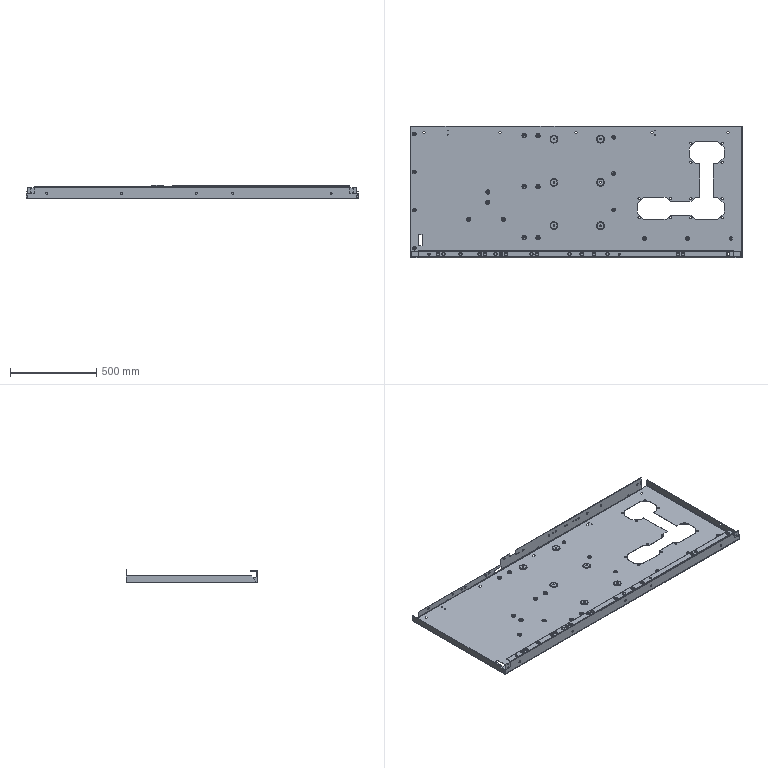Part | STEP file | 1 solid | 929 faces | box 1920 x 759 x 80 mm | volume 3915251 mm3 | plane 418 | cylinder 299 | torus 208 | spline 4 | commonest cylinder face diameters 13 x43 20.5 x42 7 x29 11 x22 4.7 x20 6.4 x20